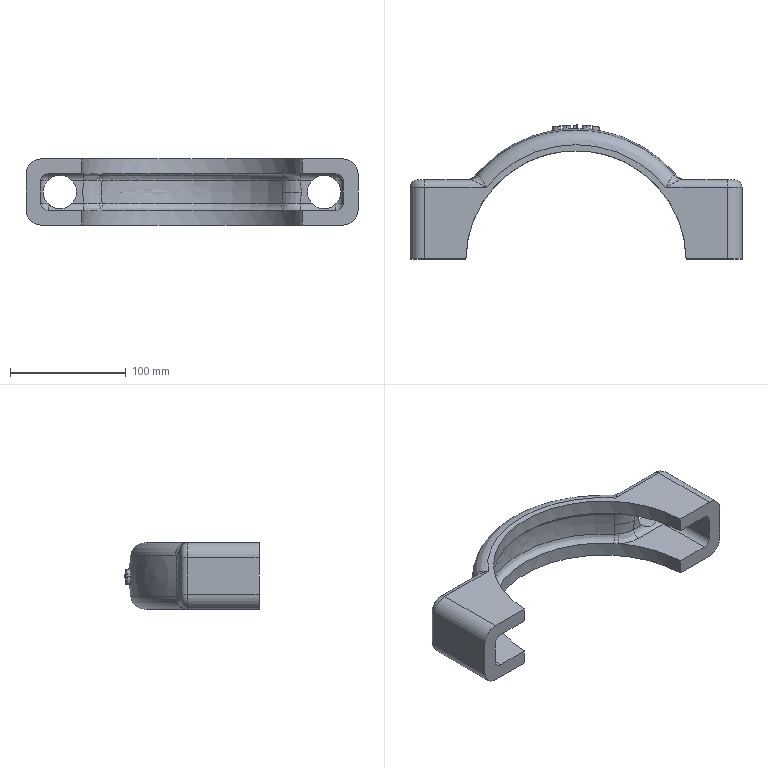Part | SolidWorks | features Fillet 6, Boss 1, Cut 1, Extrusion 1, Revolution 1, Shell 1 | 1 solid | 138 faces | box 287 x 115.887 x 57.15 mm | volume 415427 mm3 | spline 51 | plane 36 | cylinder 26 | torus 14 | sphere 11 | commonest cylinder face diameters 12.7 x16 25.4 x4 29 x4 190.5 x2